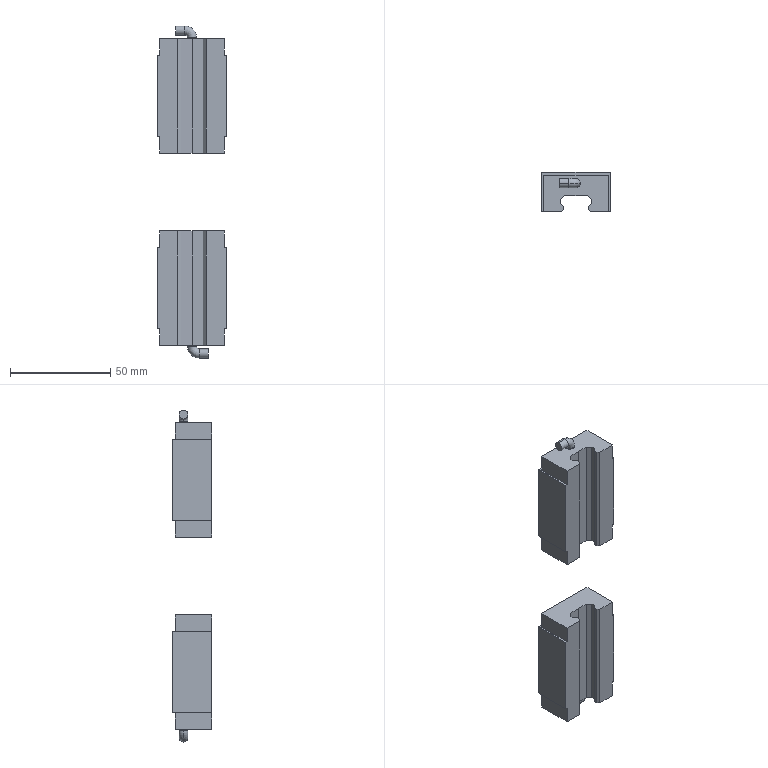Part | NX | features BREP 2 | 2 solids | 100 faces | box 34 x 19.5 x 165.7 mm | volume 60409 mm3 | plane 56 | cylinder 24 | cone 16 | torus 4 | commonest cylinder face diameters 3.3 x16 4.5 x8